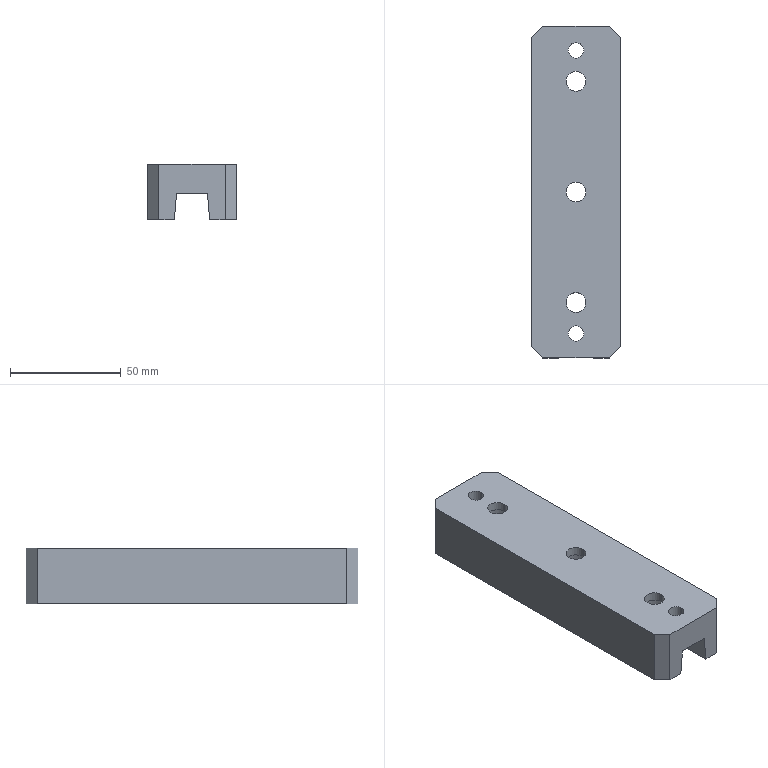Part | Creo | 1 solid | 42 faces | box 40 x 150 x 25 mm | volume 115304 mm3 | plane 26 | cylinder 16 | commonest cylinder face diameters 9 x6 15 x6 7 x4
STEP:
#1=CARTESIAN_POINT('',(0.,0.,0.));
#2=DIRECTION('',(0.,0.,1.));
#3=DIRECTION('',(1.,0.,0.));
#4=AXIS2_PLACEMENT_3D('',#1,#2,#3);
#5=CARTESIAN_POINT('',(-275.949,-119.946,-17.441));
#6=VERTEX_POINT('',#5);
#7=CARTESIAN_POINT('',(-275.949,-164.309,-17.441));
#8=VERTEX_POINT('',#7);
#9=CARTESIAN_POINT('',(-275.949,-119.946,-17.441));
#10=DIRECTION('',(0.,-1.,0.));
#11=VECTOR('',#10,44.362);
#12=LINE('',#9,#11);
#13=EDGE_CURVE('',#6,#8,#12,.T.);
#14=ORIENTED_EDGE('',*,*,#13,.F.);
#15=CARTESIAN_POINT('',(-289.849,-119.946,-17.441));
#16=VERTEX_POINT('',#15);
#17=CARTESIAN_POINT('',(-282.899,-117.127,-17.441));
#18=DIRECTION('',(0.,0.,1.));
#19=DIRECTION('',(-0.9267,-0.3758,0.));
#20=AXIS2_PLACEMENT_3D('',#17,#18,#19);
#21=CIRCLE('',#20,7.5);
#22=EDGE_CURVE('',#16,#6,#21,.T.);
#23=ORIENTED_EDGE('',*,*,#22,.F.);
#24=CARTESIAN_POINT('',(-289.849,-164.309,-17.441));
#25=VERTEX_POINT('',#24);
#26=CARTESIAN_POINT('',(-289.849,-119.946,-17.441));
#27=DIRECTION('',(0.,-1.,0.));
#28=VECTOR('',#27,44.362);
#29=LINE('',#26,#28);
#30=EDGE_CURVE('',#16,#25,#29,.T.);
#31=ORIENTED_EDGE('',*,*,#30,.T.);
#32=CARTESIAN_POINT('',(-282.899,-167.127,-17.441));
#33=DIRECTION('',(0.,0.,1.));
#34=DIRECTION('',(0.9267,0.3758,0.));
#35=AXIS2_PLACEMENT_3D('',#32,#33,#34);
#36=CIRCLE('',#35,7.5);
#37=EDGE_CURVE('',#8,#25,#36,.T.);
#38=ORIENTED_EDGE('',*,*,#37,.F.);
#39=EDGE_LOOP('',(#14,#23,#31,#38));
#40=FACE_OUTER_BOUND('',#39,.F.);
#41=CARTESIAN_POINT('',(-282.899,-167.127,-17.441));
#42=DIRECTION('',(0.,0.,1.));
#43=DIRECTION('',(1.,0.,0.));
#44=AXIS2_PLACEMENT_3D('',#41,#42,#43);
#45=PLANE('',#44);
#46=ADVANCED_FACE('',(#40),#45,.F.);
#47=CARTESIAN_POINT('',(-274.899,-92.127,-29.441));
#48=VERTEX_POINT('',#47);
#49=CARTESIAN_POINT('',(-275.949,-92.127,-17.441));
#50=VERTEX_POINT('',#49);
#51=CARTESIAN_POINT('',(-274.899,-92.127,-29.441));
#52=DIRECTION('',(-0.08716,0.,0.9962));
#53=VECTOR('',#52,12.046);
#54=LINE('',#51,#53);
#55=EDGE_CURVE('',#48,#50,#54,.T.);
#56=ORIENTED_EDGE('',*,*,#55,.T.);
#57=CARTESIAN_POINT('',(-275.949,-114.309,-17.441));
#58=VERTEX_POINT('',#57);
#59=CARTESIAN_POINT('',(-275.949,-92.127,-17.441));
#60=DIRECTION('',(0.,-1.,0.));
#61=VECTOR('',#60,22.181);
#62=LINE('',#59,#61);
#63=EDGE_CURVE('',#50,#58,#62,.T.);
#64=ORIENTED_EDGE('',*,*,#63,.T.);
#65=CARTESIAN_POINT('',(-275.949,-114.309,-17.441));
#66=DIRECTION('',(0.,-1.,0.));
#67=VECTOR('',#66,5.638);
#68=LINE('',#65,#67);
#69=EDGE_CURVE('',#58,#6,#68,.T.);
#70=ORIENTED_EDGE('',*,*,#69,.T.);
#71=ORIENTED_EDGE('',*,*,#13,.T.);
#72=CARTESIAN_POINT('',(-275.949,-169.946,-17.441));
#73=VERTEX_POINT('',#72);
#74=CARTESIAN_POINT('',(-275.949,-164.309,-17.441));
#75=DIRECTION('',(0.,-1.,0.));
#76=VECTOR('',#75,5.638);
#77=LINE('',#74,#76);
#78=EDGE_CURVE('',#8,#73,#77,.T.);
#79=ORIENTED_EDGE('',*,*,#78,.T.);
#80=CARTESIAN_POINT('',(-275.949,-214.309,-17.441));
#81=VERTEX_POINT('',#80);
#82=CARTESIAN_POINT('',(-275.949,-169.946,-17.441));
#83=DIRECTION('',(0.,-1.,0.));
#84=VECTOR('',#83,44.362);
#85=LINE('',#82,#84);
#86=EDGE_CURVE('',#73,#81,#85,.T.);
#87=ORIENTED_EDGE('',*,*,#86,.T.);
#88=CARTESIAN_POINT('',(-275.949,-219.946,-17.441));
#89=VERTEX_POINT('',#88);
#90=CARTESIAN_POINT('',(-275.949,-214.309,-17.441));
#91=DIRECTION('',(0.,-1.,0.));
#92=VECTOR('',#91,5.638);
#93=LINE('',#90,#92);
#94=EDGE_CURVE('',#81,#89,#93,.T.);
#95=ORIENTED_EDGE('',*,*,#94,.T.);
#96=CARTESIAN_POINT('',(-275.949,-242.127,-17.441));
#97=VERTEX_POINT('',#96);
#98=CARTESIAN_POINT('',(-275.949,-219.946,-17.441));
#99=DIRECTION('',(0.,-1.,0.));
#100=VECTOR('',#99,22.181);
#101=LINE('',#98,#100);
#102=EDGE_CURVE('',#89,#97,#101,.T.);
#103=ORIENTED_EDGE('',*,*,#102,.T.);
#104=CARTESIAN_POINT('',(-274.899,-242.127,-29.441));
#105=VERTEX_POINT('',#104);
#106=CARTESIAN_POINT('',(-275.949,-242.127,-17.441));
#107=DIRECTION('',(0.08716,0.,-0.9962));
#108=VECTOR('',#107,12.046);
#109=LINE('',#106,#108);
#110=EDGE_CURVE('',#97,#105,#109,.T.);
#111=ORIENTED_EDGE('',*,*,#110,.T.);
#112=CARTESIAN_POINT('',(-274.899,-92.127,-29.441));
#113=DIRECTION('',(0.,-1.,0.));
#114=VECTOR('',#113,150.);
#115=LINE('',#112,#114);
#116=EDGE_CURVE('',#48,#105,#115,.T.);
#117=ORIENTED_EDGE('',*,*,#116,.F.);
#118=EDGE_LOOP('',(#56,#64,#70,#71,#79,#87,#95,#103,#111,#117));
#119=FACE_OUTER_BOUND('',#118,.F.);
#120=CARTESIAN_POINT('',(-274.899,-92.127,-29.441));
#121=DIRECTION('',(-0.9962,0.,-0.08716));
#122=DIRECTION('',(-0.08716,0.,0.9962));
#123=AXIS2_PLACEMENT_3D('',#120,#121,#122);
#124=PLANE('',#123);
#125=ADVANCED_FACE('',(#119),#124,.T.);
#126=CARTESIAN_POINT('',(-289.849,-92.127,-17.441));
#127=VERTEX_POINT('',#126);
#128=CARTESIAN_POINT('',(-290.899,-92.127,-29.441));
#129=VERTEX_POINT('',#128);
#130=CARTESIAN_POINT('',(-289.849,-92.127,-17.441));
#131=DIRECTION('',(-0.08716,0.,-0.9962));
#132=VECTOR('',#131,12.046);
#133=LINE('',#130,#132);
#134=EDGE_CURVE('',#127,#129,#133,.T.);
#135=ORIENTED_EDGE('',*,*,#134,.F.);
#136=CARTESIAN_POINT('',(-289.849,-92.127,-17.441));
#137=DIRECTION('',(1.,0.,0.));
#138=VECTOR('',#137,13.9);
#139=LINE('',#136,#138);
#140=EDGE_CURVE('',#127,#50,#139,.T.);
#141=ORIENTED_EDGE('',*,*,#140,.T.);
#142=ORIENTED_EDGE('',*,*,#55,.F.);
#143=CARTESIAN_POINT('',(-267.899,-92.127,-29.441));
#144=VERTEX_POINT('',#143);
#145=CARTESIAN_POINT('',(-274.899,-92.127,-29.441));
#146=DIRECTION('',(1.,0.,0.));
#147=VECTOR('',#146,7.);
#148=LINE('',#145,#147);
#149=EDGE_CURVE('',#48,#144,#148,.T.);
#150=ORIENTED_EDGE('',*,*,#149,.T.);
#151=CARTESIAN_POINT('',(-267.899,-92.127,-4.441));
#152=VERTEX_POINT('',#151);
#153=CARTESIAN_POINT('',(-267.899,-92.127,-4.441));
#154=DIRECTION('',(0.,0.,-1.));
#155=VECTOR('',#154,25.);
#156=LINE('',#153,#155);
#157=EDGE_CURVE('',#152,#144,#156,.T.);
#158=ORIENTED_EDGE('',*,*,#157,.F.);
#159=CARTESIAN_POINT('',(-297.899,-92.127,-4.441));
#160=VERTEX_POINT('',#159);
#161=CARTESIAN_POINT('',(-297.899,-92.127,-4.441));
#162=DIRECTION('',(1.,0.,0.));
#163=VECTOR('',#162,30.);
#164=LINE('',#161,#163);
#165=EDGE_CURVE('',#160,#152,#164,.T.);
#166=ORIENTED_EDGE('',*,*,#165,.F.);
#167=CARTESIAN_POINT('',(-297.899,-92.127,-29.441));
#168=VERTEX_POINT('',#167);
#169=CARTESIAN_POINT('',(-297.899,-92.127,-29.441));
#170=DIRECTION('',(0.,0.,1.));
#171=VECTOR('',#170,25.);
#172=LINE('',#169,#171);
#173=EDGE_CURVE('',#168,#160,#172,.T.);
#174=ORIENTED_EDGE('',*,*,#173,.F.);
#175=CARTESIAN_POINT('',(-297.899,-92.127,-29.441));
#176=DIRECTION('',(1.,0.,0.));
#177=VECTOR('',#176,7.);
#178=LINE('',#175,#177);
#179=EDGE_CURVE('',#168,#129,#178,.T.);
#180=ORIENTED_EDGE('',*,*,#179,.T.);
#181=EDGE_LOOP('',(#135,#141,#142,#150,#158,#166,#174,#180));
#182=FACE_OUTER_BOUND('',#181,.F.);
#183=CARTESIAN_POINT('',(-262.899,-92.127,-4.441));
#184=DIRECTION('',(0.,1.,0.));
#185=DIRECTION('',(0.,0.,1.));
#186=AXIS2_PLACEMENT_3D('',#183,#184,#185);
#187=PLANE('',#186);
#188=ADVANCED_FACE('',(#182),#187,.T.);
#189=ORIENTED_EDGE('',*,*,#134,.T.);
#190=CARTESIAN_POINT('',(-290.899,-242.127,-29.441));
#191=VERTEX_POINT('',#190);
#192=CARTESIAN_POINT('',(-290.899,-92.127,-29.441));
#193=DIRECTION('',(0.,-1.,0.));
#194=VECTOR('',#193,150.);
#195=LINE('',#192,#194);
#196=EDGE_CURVE('',#129,#191,#195,.T.);
#197=ORIENTED_EDGE('',*,*,#196,.T.);
#198=CARTESIAN_POINT('',(-289.849,-242.127,-17.441));
#199=VERTEX_POINT('',#198);
#200=CARTESIAN_POINT('',(-290.899,-242.127,-29.441));
#201=DIRECTION('',(0.08716,0.,0.9962));
#202=VECTOR('',#201,12.046);
#203=LINE('',#200,#202);
#204=EDGE_CURVE('',#191,#199,#203,.T.);
#205=ORIENTED_EDGE('',*,*,#204,.T.);
#206=CARTESIAN_POINT('',(-289.849,-219.946,-17.441));
#207=VERTEX_POINT('',#206);
#208=CARTESIAN_POINT('',(-289.849,-219.946,-17.441));
#209=DIRECTION('',(0.,-1.,0.));
#210=VECTOR('',#209,22.181);
#211=LINE('',#208,#210);
#212=EDGE_CURVE('',#207,#199,#211,.T.);
#213=ORIENTED_EDGE('',*,*,#212,.F.);
#214=CARTESIAN_POINT('',(-289.849,-214.309,-17.441));
#215=VERTEX_POINT('',#214);
#216=CARTESIAN_POINT('',(-289.849,-214.309,-17.441));
#217=DIRECTION('',(0.,-1.,0.));
#218=VECTOR('',#217,5.638);
#219=LINE('',#216,#218);
#220=EDGE_CURVE('',#215,#207,#219,.T.);
#221=ORIENTED_EDGE('',*,*,#220,.F.);
#222=CARTESIAN_POINT('',(-289.849,-169.946,-17.441));
#223=VERTEX_POINT('',#222);
#224=CARTESIAN_POINT('',(-289.849,-169.946,-17.441));
#225=DIRECTION('',(0.,-1.,0.));
#226=VECTOR('',#225,44.362);
#227=LINE('',#224,#226);
#228=EDGE_CURVE('',#223,#215,#227,.T.);
#229=ORIENTED_EDGE('',*,*,#228,.F.);
#230=CARTESIAN_POINT('',(-289.849,-164.309,-17.441));
#231=DIRECTION('',(0.,-1.,0.));
#232=VECTOR('',#231,5.638);
#233=LINE('',#230,#232);
#234=EDGE_CURVE('',#25,#223,#233,.T.);
#235=ORIENTED_EDGE('',*,*,#234,.F.);
#236=ORIENTED_EDGE('',*,*,#30,.F.);
#237=CARTESIAN_POINT('',(-289.849,-114.309,-17.441));
#238=VERTEX_POINT('',#237);
#239=CARTESIAN_POINT('',(-289.849,-114.309,-17.441));
#240=DIRECTION('',(0.,-1.,0.));
#241=VECTOR('',#240,5.638);
#242=LINE('',#239,#241);
#243=EDGE_CURVE('',#238,#16,#242,.T.);
#244=ORIENTED_EDGE('',*,*,#243,.F.);
#245=CARTESIAN_POINT('',(-289.849,-92.127,-17.441));
#246=DIRECTION('',(0.,-1.,0.));
#247=VECTOR('',#246,22.181);
#248=LINE('',#245,#247);
#249=EDGE_CURVE('',#127,#238,#248,.T.);
#250=ORIENTED_EDGE('',*,*,#249,.F.);
#251=EDGE_LOOP('',(#189,#197,#205,#213,#221,#229,#235,#236,#244,#250));
#252=FACE_OUTER_BOUND('',#251,.F.);
#253=CARTESIAN_POINT('',(-290.899,-92.127,-29.441));
#254=DIRECTION('',(0.9962,0.,-0.08716));
#255=DIRECTION('',(-0.08716,0.,-0.9962));
#256=AXIS2_PLACEMENT_3D('',#253,#254,#255);
#257=PLANE('',#256);
#258=ADVANCED_FACE('',(#252),#257,.T.);
#259=CARTESIAN_POINT('',(-297.899,-242.127,-29.441));
#260=VERTEX_POINT('',#259);
#261=CARTESIAN_POINT('',(-290.899,-242.127,-29.441));
#262=DIRECTION('',(-1.,0.,0.));
#263=VECTOR('',#262,7.);
#264=LINE('',#261,#263);
#265=EDGE_CURVE('',#191,#260,#264,.T.);
#266=ORIENTED_EDGE('',*,*,#265,.F.);
#267=ORIENTED_EDGE('',*,*,#196,.F.);
#268=ORIENTED_EDGE('',*,*,#179,.F.);
#269=CARTESIAN_POINT('',(-302.899,-97.127,-29.441));
#270=VERTEX_POINT('',#269);
#271=CARTESIAN_POINT('',(-302.899,-97.127,-29.441));
#272=DIRECTION('',(0.7071,0.7071,0.));
#273=VECTOR('',#272,7.071);
#274=LINE('',#271,#273);
#275=EDGE_CURVE('',#270,#168,#274,.T.);
#276=ORIENTED_EDGE('',*,*,#275,.F.);
#277=CARTESIAN_POINT('',(-302.899,-237.127,-29.441));
#278=VERTEX_POINT('',#277);
#279=CARTESIAN_POINT('',(-302.899,-237.127,-29.441));
#280=DIRECTION('',(0.,1.,0.));
#281=VECTOR('',#280,140.);
#282=LINE('',#279,#281);
#283=EDGE_CURVE('',#278,#270,#282,.T.);
#284=ORIENTED_EDGE('',*,*,#283,.F.);
#285=CARTESIAN_POINT('',(-297.899,-242.127,-29.441));
#286=DIRECTION('',(-0.7071,0.7071,0.));
#287=VECTOR('',#286,7.071);
#288=LINE('',#285,#287);
#289=EDGE_CURVE('',#260,#278,#288,.T.);
#290=ORIENTED_EDGE('',*,*,#289,.F.);
#291=EDGE_LOOP('',(#266,#267,#268,#276,#284,#290));
#292=FACE_OUTER_BOUND('',#291,.F.);
#293=CARTESIAN_POINT('',(-302.899,-242.127,-29.441));
#294=DIRECTION('',(0.,0.,1.));
#295=DIRECTION('',(1.,0.,0.));
#296=AXIS2_PLACEMENT_3D('',#293,#294,#295);
#297=PLANE('',#296);
#298=ADVANCED_FACE('',(#292),#297,.F.);
#299=ORIENTED_EDGE('',*,*,#204,.F.);
#300=ORIENTED_EDGE('',*,*,#265,.T.);
#301=CARTESIAN_POINT('',(-297.899,-242.127,-4.441));
#302=VERTEX_POINT('',#301);
#303=CARTESIAN_POINT('',(-297.899,-242.127,-4.441));
#304=DIRECTION('',(0.,0.,-1.));
#305=VECTOR('',#304,25.);
#306=LINE('',#303,#305);
#307=EDGE_CURVE('',#302,#260,#306,.T.);
#308=ORIENTED_EDGE('',*,*,#307,.F.);
#309=CARTESIAN_POINT('',(-267.899,-242.127,-4.441));
#310=VERTEX_POINT('',#309);
#311=CARTESIAN_POINT('',(-267.899,-242.127,-4.441));
#312=DIRECTION('',(-1.,0.,0.));
#313=VECTOR('',#312,30.);
#314=LINE('',#311,#313);
#315=EDGE_CURVE('',#310,#302,#314,.T.);
#316=ORIENTED_EDGE('',*,*,#315,.F.);
#317=CARTESIAN_POINT('',(-267.899,-242.127,-29.441));
#318=VERTEX_POINT('',#317);
#319=CARTESIAN_POINT('',(-267.899,-242.127,-29.441));
#320=DIRECTION('',(0.,0.,1.));
#321=VECTOR('',#320,25.);
#322=LINE('',#319,#321);
#323=EDGE_CURVE('',#318,#310,#322,.T.);
#324=ORIENTED_EDGE('',*,*,#323,.F.);
#325=CARTESIAN_POINT('',(-267.899,-242.127,-29.441));
#326=DIRECTION('',(-1.,0.,0.));
#327=VECTOR('',#326,7.);
#328=LINE('',#325,#327);
#329=EDGE_CURVE('',#318,#105,#328,.T.);
#330=ORIENTED_EDGE('',*,*,#329,.T.);
#331=ORIENTED_EDGE('',*,*,#110,.F.);
#332=CARTESIAN_POINT('',(-275.949,-242.127,-17.441));
#333=DIRECTION('',(-1.,0.,0.));
#334=VECTOR('',#333,13.9);
#335=LINE('',#332,#334);
#336=EDGE_CURVE('',#97,#199,#335,.T.);
#337=ORIENTED_EDGE('',*,*,#336,.T.);
#338=EDGE_LOOP('',(#299,#300,#308,#316,#324,#330,#331,#337));
#339=FACE_OUTER_BOUND('',#338,.F.);
#340=CARTESIAN_POINT('',(-302.899,-242.127,-4.441));
#341=DIRECTION('',(0.,-1.,0.));
#342=DIRECTION('',(0.,0.,-1.));
#343=AXIS2_PLACEMENT_3D('',#340,#341,#342);
#344=PLANE('',#343);
#345=ADVANCED_FACE('',(#339),#344,.T.);
#346=CARTESIAN_POINT('',(-302.899,-237.127,-4.441));
#347=VERTEX_POINT('',#346);
#348=CARTESIAN_POINT('',(-302.899,-237.127,-4.441));
#349=DIRECTION('',(0.7071,-0.7071,0.));
#350=VECTOR('',#349,7.071);
#351=LINE('',#348,#350);
#352=EDGE_CURVE('',#347,#302,#351,.T.);
#353=ORIENTED_EDGE('',*,*,#352,.T.);
#354=ORIENTED_EDGE('',*,*,#307,.T.);
#355=ORIENTED_EDGE('',*,*,#289,.T.);
#356=CARTESIAN_POINT('',(-302.899,-237.127,-29.441));
#357=DIRECTION('',(0.,0.,1.));
#358=VECTOR('',#357,25.);
#359=LINE('',#356,#358);
#360=EDGE_CURVE('',#278,#347,#359,.T.);
#361=ORIENTED_EDGE('',*,*,#360,.T.);
#362=EDGE_LOOP('',(#353,#354,#355,#361));
#363=FACE_OUTER_BOUND('',#362,.F.);
#364=CARTESIAN_POINT('',(-302.899,-237.127,-4.441));
#365=DIRECTION('',(0.7071,0.7071,0.));
#366=DIRECTION('',(-0.7071,0.7071,0.));
#367=AXIS2_PLACEMENT_3D('',#364,#365,#366);
#368=PLANE('',#367);
#369=ADVANCED_FACE('',(#363),#368,.F.);
#370=CARTESIAN_POINT('',(-302.899,-97.127,-4.441));
#371=VERTEX_POINT('',#370);
#372=CARTESIAN_POINT('',(-302.899,-237.127,-4.441));
#373=DIRECTION('',(0.,1.,0.));
#374=VECTOR('',#373,140.);
#375=LINE('',#372,#374);
#376=EDGE_CURVE('',#347,#371,#375,.T.);
#377=ORIENTED_EDGE('',*,*,#376,.T.);
#378=CARTESIAN_POINT('',(-297.899,-92.127,-4.441));
#379=DIRECTION('',(-0.7071,-0.7071,0.));
#380=VECTOR('',#379,7.071);
#381=LINE('',#378,#380);
#382=EDGE_CURVE('',#160,#371,#381,.T.);
#383=ORIENTED_EDGE('',*,*,#382,.F.);
#384=ORIENTED_EDGE('',*,*,#165,.T.);
#385=CARTESIAN_POINT('',(-262.899,-97.127,-4.441));
#386=VERTEX_POINT('',#385);
#387=CARTESIAN_POINT('',(-262.899,-97.127,-4.441));
#388=DIRECTION('',(-0.7071,0.7071,0.));
#389=VECTOR('',#388,7.071);
#390=LINE('',#387,#389);
#391=EDGE_CURVE('',#386,#152,#390,.T.);
#392=ORIENTED_EDGE('',*,*,#391,.F.);
#393=CARTESIAN_POINT('',(-262.899,-237.127,-4.441));
#394=VERTEX_POINT('',#393);
#395=CARTESIAN_POINT('',(-262.899,-97.127,-4.441));
#396=DIRECTION('',(0.,-1.,0.));
#397=VECTOR('',#396,140.);
#398=LINE('',#395,#397);
#399=EDGE_CURVE('',#386,#394,#398,.T.);
#400=ORIENTED_EDGE('',*,*,#399,.T.);
#401=CARTESIAN_POINT('',(-267.899,-242.127,-4.441));
#402=DIRECTION('',(0.7071,0.7071,0.));
#403=VECTOR('',#402,7.071);
#404=LINE('',#401,#403);
#405=EDGE_CURVE('',#310,#394,#404,.T.);
#406=ORIENTED_EDGE('',*,*,#405,.F.);
#407=ORIENTED_EDGE('',*,*,#315,.T.);
#408=ORIENTED_EDGE('',*,*,#352,.F.);
#409=EDGE_LOOP('',(#377,#383,#384,#392,#400,#406,#407,#408));
#410=FACE_OUTER_BOUND('',#409,.F.);
#411=CARTESIAN_POINT('',(-278.399,-167.127,-4.441));
#412=VERTEX_POINT('',#411);
#413=CARTESIAN_POINT('',(-287.399,-167.127,-4.441));
#414=VERTEX_POINT('',#413);
#415=CARTESIAN_POINT('',(-282.899,-167.127,-4.441));
#416=DIRECTION('',(0.,0.,-1.));
#417=DIRECTION('',(1.,0.,0.));
#418=AXIS2_PLACEMENT_3D('',#415,#416,#417);
#419=CIRCLE('',#418,4.5);
#420=EDGE_CURVE('',#412,#414,#419,.T.);
#421=ORIENTED_EDGE('',*,*,#420,.F.);
#422=CARTESIAN_POINT('',(-282.899,-167.127,-4.441));
#423=DIRECTION('',(0.,0.,-1.));
#424=DIRECTION('',(-1.,0.,0.));
#425=AXIS2_PLACEMENT_3D('',#422,#423,#424);
#426=CIRCLE('',#425,4.5);
#427=EDGE_CURVE('',#414,#412,#426,.T.);
#428=ORIENTED_EDGE('',*,*,#427,.F.);
#429=EDGE_LOOP('',(#421,#428));
#430=FACE_BOUND('',#429,.F.);
#431=CARTESIAN_POINT('',(-278.399,-217.127,-4.441));
#432=VERTEX_POINT('',#431);
#433=CARTESIAN_POINT('',(-287.399,-217.127,-4.441));
#434=VERTEX_POINT('',#433);
#435=CARTESIAN_POINT('',(-282.899,-217.127,-4.441));
#436=DIRECTION('',(0.,0.,-1.));
#437=DIRECTION('',(1.,0.,0.));
#438=AXIS2_PLACEMENT_3D('',#435,#436,#437);
#439=CIRCLE('',#438,4.5);
#440=EDGE_CURVE('',#432,#434,#439,.T.);
#441=ORIENTED_EDGE('',*,*,#440,.F.);
#442=CARTESIAN_POINT('',(-282.899,-217.127,-4.441));
#443=DIRECTION('',(0.,0.,-1.));
#444=DIRECTION('',(-1.,0.,0.));
#445=AXIS2_PLACEMENT_3D('',#442,#443,#444);
#446=CIRCLE('',#445,4.5);
#447=EDGE_CURVE('',#434,#432,#446,.T.);
#448=ORIENTED_EDGE('',*,*,#447,.F.);
#449=EDGE_LOOP('',(#441,#448));
#450=FACE_BOUND('',#449,.F.);
#451=CARTESIAN_POINT('',(-279.399,-103.127,-4.441));
#452=VERTEX_POINT('',#451);
#453=CARTESIAN_POINT('',(-286.399,-103.127,-4.441));
#454=VERTEX_POINT('',#453);
#455=CARTESIAN_POINT('',(-282.899,-103.127,-4.441));
#456=DIRECTION('',(0.,0.,-1.));
#457=DIRECTION('',(1.,0.,0.));
#458=AXIS2_PLACEMENT_3D('',#455,#456,#457);
#459=CIRCLE('',#458,3.5);
#460=EDGE_CURVE('',#452,#454,#459,.T.);
#461=ORIENTED_EDGE('',*,*,#460,.F.);
#462=CARTESIAN_POINT('',(-282.899,-103.127,-4.441));
#463=DIRECTION('',(0.,0.,-1.));
#464=DIRECTION('',(-1.,0.,0.));
#465=AXIS2_PLACEMENT_3D('',#462,#463,#464);
#466=CIRCLE('',#465,3.5);
#467=EDGE_CURVE('',#454,#452,#466,.T.);
#468=ORIENTED_EDGE('',*,*,#467,.F.);
#469=EDGE_LOOP('',(#461,#468));
#470=FACE_BOUND('',#469,.F.);
#471=CARTESIAN_POINT('',(-278.399,-117.127,-4.441));
#472=VERTEX_POINT('',#471);
#473=CARTESIAN_POINT('',(-287.399,-117.127,-4.441));
#474=VERTEX_POINT('',#473);
#475=CARTESIAN_POINT('',(-282.899,-117.127,-4.441));
#476=DIRECTION('',(0.,0.,-1.));
#477=DIRECTION('',(1.,0.,0.));
#478=AXIS2_PLACEMENT_3D('',#475,#476,#477);
#479=CIRCLE('',#478,4.5);
#480=EDGE_CURVE('',#472,#474,#479,.T.);
#481=ORIENTED_EDGE('',*,*,#480,.F.);
#482=CARTESIAN_POINT('',(-282.899,-117.127,-4.441));
#483=DIRECTION('',(0.,0.,-1.));
#484=DIRECTION('',(-1.,0.,0.));
#485=AXIS2_PLACEMENT_3D('',#482,#483,#484);
#486=CIRCLE('',#485,4.5);
#487=EDGE_CURVE('',#474,#472,#486,.T.);
#488=ORIENTED_EDGE('',*,*,#487,.F.);
#489=EDGE_LOOP('',(#481,#488));
#490=FACE_BOUND('',#489,.F.);
#491=CARTESIAN_POINT('',(-279.399,-231.127,-4.441));
#492=VERTEX_POINT('',#491);
#493=CARTESIAN_POINT('',(-286.399,-231.127,-4.441));
#494=VERTEX_POINT('',#493);
#495=CARTESIAN_POINT('',(-282.899,-231.127,-4.441));
#496=DIRECTION('',(0.,0.,-1.));
#497=DIRECTION('',(1.,0.,0.));
#498=AXIS2_PLACEMENT_3D('',#495,#496,#497);
#499=CIRCLE('',#498,3.5);
#500=EDGE_CURVE('',#492,#494,#499,.T.);
#501=ORIENTED_EDGE('',*,*,#500,.F.);
#502=CARTESIAN_POINT('',(-282.899,-231.127,-4.441));
#503=DIRECTION('',(0.,0.,-1.));
#504=DIRECTION('',(-1.,0.,0.));
#505=AXIS2_PLACEMENT_3D('',#502,#503,#504);
#506=CIRCLE('',#505,3.5);
#507=EDGE_CURVE('',#494,#492,#506,.T.);
#508=ORIENTED_EDGE('',*,*,#507,.F.);
#509=EDGE_LOOP('',(#501,#508));
#510=FACE_BOUND('',#509,.F.);
#511=CARTESIAN_POINT('',(-302.899,-242.127,-4.441));
#512=DIRECTION('',(0.,0.,1.));
#513=DIRECTION('',(1.,0.,0.));
#514=AXIS2_PLACEMENT_3D('',#511,#512,#513);
#515=PLANE('',#514);
#516=ADVANCED_FACE('',(#410,#430,#450,#470,#490,#510),#515,.T.);
#517=ORIENTED_EDGE('',*,*,#480,.T.);
#518=CARTESIAN_POINT('',(-287.399,-117.127,-8.441));
#519=VERTEX_POINT('',#518);
#520=CARTESIAN_POINT('',(-287.399,-117.127,-4.441));
#521=DIRECTION('',(0.,0.,-1.));
#522=VECTOR('',#521,4.);
#523=LINE('',#520,#522);
#524=EDGE_CURVE('',#474,#519,#523,.T.);
#525=ORIENTED_EDGE('',*,*,#524,.T.);
#526=CARTESIAN_POINT('',(-278.399,-117.127,-8.441));
#527=VERTEX_POINT('',#526);
#528=CARTESIAN_POINT('',(-282.899,-117.127,-8.441));
#529=DIRECTION('',(0.,0.,1.));
#530=DIRECTION('',(-1.,0.,0.));
#531=AXIS2_PLACEMENT_3D('',#528,#529,#530);
#532=CIRCLE('',#531,4.5);
#533=EDGE_CURVE('',#519,#527,#532,.T.);
#534=ORIENTED_EDGE('',*,*,#533,.T.);
#535=CARTESIAN_POINT('',(-278.399,-117.127,-4.441));
#536=DIRECTION('',(0.,0.,-1.));
#537=VECTOR('',#536,4.);
#538=LINE('',#535,#537);
#539=EDGE_CURVE('',#472,#527,#538,.T.);
#540=ORIENTED_EDGE('',*,*,#539,.F.);
#541=EDGE_LOOP('',(#517,#525,#534,#540));
#542=FACE_OUTER_BOUND('',#541,.F.);
#543=CARTESIAN_POINT('',(-282.899,-117.127,26.559));
#544=DIRECTION('',(0.,0.,-1.));
#545=DIRECTION('',(-1.,0.,0.));
#546=AXIS2_PLACEMENT_3D('',#543,#544,#545);
#547=CYLINDRICAL_SURFACE('',#546,4.5);
#548=ADVANCED_FACE('',(#542),#547,.F.);
#549=ORIENTED_EDGE('',*,*,#487,.T.);
#550=ORIENTED_EDGE('',*,*,#539,.T.);
#551=CARTESIAN_POINT('',(-282.899,-117.127,-8.441));
#552=DIRECTION('',(0.,0.,1.));
#553=DIRECTION('',(1.,0.,0.));
#554=AXIS2_PLACEMENT_3D('',#551,#552,#553);
#555=CIRCLE('',#554,4.5);
#556=EDGE_CURVE('',#527,#519,#555,.T.);
#557=ORIENTED_EDGE('',*,*,#556,.T.);
#558=ORIENTED_EDGE('',*,*,#524,.F.);
#559=EDGE_LOOP('',(#549,#550,#557,#558));
#560=FACE_OUTER_BOUND('',#559,.F.);
#561=CARTESIAN_POINT('',(-282.899,-117.127,26.559));
#562=DIRECTION('',(0.,0.,-1.));
#563=DIRECTION('',(-1.,0.,0.));
#564=AXIS2_PLACEMENT_3D('',#561,#562,#563);
#565=CYLINDRICAL_SURFACE('',#564,4.5);
#566=ADVANCED_FACE('',(#560),#565,.F.);
#567=CARTESIAN_POINT('',(-290.399,-117.127,-8.441));
#568=VERTEX_POINT('',#567);
#569=CARTESIAN_POINT('',(-275.399,-117.127,-8.441));
#570=VERTEX_POINT('',#569);
#571=CARTESIAN_POINT('',(-282.899,-117.127,-8.441));
#572=DIRECTION('',(0.,0.,-1.));
#573=DIRECTION('',(-1.,0.,0.));
#574=AXIS2_PLACEMENT_3D('',#571,#572,#573);
#575=CIRCLE('',#574,7.5);
#576=EDGE_CURVE('',#568,#570,#575,.T.);
#577=ORIENTED_EDGE('',*,*,#576,.F.);
#578=CARTESIAN_POINT('',(-282.899,-117.127,-8.441));
#579=DIRECTION('',(0.,0.,-1.));
#580=DIRECTION('',(1.,0.,0.));
#581=AXIS2_PLACEMENT_3D('',#578,#579,#580);
#582=CIRCLE('',#581,7.5);
#583=EDGE_CURVE('',#570,#568,#582,.T.);
#584=ORIENTED_EDGE('',*,*,#583,.F.);
#585=EDGE_LOOP('',(#577,#584));
#586=FACE_OUTER_BOUND('',#585,.F.);
#587=ORIENTED_EDGE('',*,*,#533,.F.);
#588=ORIENTED_EDGE('',*,*,#556,.F.);
#589=EDGE_LOOP('',(#587,#588));
#590=FACE_BOUND('',#589,.F.);
#591=CARTESIAN_POINT('',(-282.899,-117.127,-8.441));
#592=DIRECTION('',(0.,0.,-1.));
#593=DIRECTION('',(-1.,0.,0.));
#594=AXIS2_PLACEMENT_3D('',#591,#592,#593);
#595=PLANE('',#594);
#596=ADVANCED_FACE('',(#586,#590),#595,.T.);
#597=ORIENTED_EDGE('',*,*,#576,.T.);
#598=CARTESIAN_POINT('',(-275.399,-117.127,-17.441));
#599=VERTEX_POINT('',#598);
#600=CARTESIAN_POINT('',(-275.399,-117.127,-8.441));
#601=DIRECTION('',(0.,0.,-1.));
#602=VECTOR('',#601,9.);
#603=LINE('',#600,#602);
#604=EDGE_CURVE('',#570,#599,#603,.T.);
#605=ORIENTED_EDGE('',*,*,#604,.T.);
#606=CARTESIAN_POINT('',(-282.899,-117.127,-17.441));
#607=DIRECTION('',(0.,0.,1.));
#608=DIRECTION('',(1.,0.,0.));
#609=AXIS2_PLACEMENT_3D('',#606,#607,#608);
#610=CIRCLE('',#609,7.5);
#611=EDGE_CURVE('',#599,#58,#610,.T.);
#612=ORIENTED_EDGE('',*,*,#611,.T.);
#613=CARTESIAN_POINT('',(-282.899,-117.127,-17.441));
#614=DIRECTION('',(0.,0.,1.));
#615=DIRECTION('',(0.9267,0.3758,0.));
#616=AXIS2_PLACEMENT_3D('',#613,#614,#615);
#617=CIRCLE('',#616,7.5);
#618=EDGE_CURVE('',#58,#238,#617,.T.);
#619=ORIENTED_EDGE('',*,*,#618,.T.);
#620=CARTESIAN_POINT('',(-290.399,-117.127,-17.441));
#621=VERTEX_POINT('',#620);
#622=CARTESIAN_POINT('',(-282.899,-117.127,-17.441));
#623=DIRECTION('',(0.,0.,1.));
#624=DIRECTION('',(-0.9267,0.3758,0.));
#625=AXIS2_PLACEMENT_3D('',#622,#623,#624);
#626=CIRCLE('',#625,7.5);
#627=EDGE_CURVE('',#238,#621,#626,.T.);
#628=ORIENTED_EDGE('',*,*,#627,.T.);
#629=CARTESIAN_POINT('',(-290.399,-117.127,-8.441));
#630=DIRECTION('',(0.00000035,0.,-1.));
#631=VECTOR('',#630,9.);
#632=LINE('',#629,#631);
#633=EDGE_CURVE('',#568,#621,#632,.T.);
#634=ORIENTED_EDGE('',*,*,#633,.F.);
#635=EDGE_LOOP('',(#597,#605,#612,#619,#628,#634));
#636=FACE_OUTER_BOUND('',#635,.F.);
#637=CARTESIAN_POINT('',(-282.899,-117.127,-8.441));
#638=DIRECTION('',(0.,0.,-1.));
#639=DIRECTION('',(-1.,0.,0.));
#640=AXIS2_PLACEMENT_3D('',#637,#638,#639);
#641=CYLINDRICAL_SURFACE('',#640,7.5);
#642=ADVANCED_FACE('',(#636),#641,.F.);
#643=ORIENTED_EDGE('',*,*,#583,.T.);
#644=ORIENTED_EDGE('',*,*,#633,.T.);
#645=CARTESIAN_POINT('',(-282.899,-117.127,-17.441));
#646=DIRECTION('',(0.,0.,1.));
#647=DIRECTION('',(-1.,0.,0.));
#648=AXIS2_PLACEMENT_3D('',#645,#646,#647);
#649=CIRCLE('',#648,7.5);
#650=EDGE_CURVE('',#621,#16,#649,.T.);
#651=ORIENTED_EDGE('',*,*,#650,.T.);
#652=ORIENTED_EDGE('',*,*,#22,.T.);
#653=CARTESIAN_POINT('',(-282.899,-117.127,-17.441));
#654=DIRECTION('',(0.,0.,1.));
#655=DIRECTION('',(0.9267,-0.3758,0.));
#656=AXIS2_PLACEMENT_3D('',#653,#654,#655);
#657=CIRCLE('',#656,7.5);
#658=EDGE_CURVE('',#6,#599,#657,.T.);
#659=ORIENTED_EDGE('',*,*,#658,.T.);
#660=ORIENTED_EDGE('',*,*,#604,.F.);
#661=EDGE_LOOP('',(#643,#644,#651,#652,#659,#660));
#662=FACE_OUTER_BOUND('',#661,.F.);
#663=CARTESIAN_POINT('',(-282.899,-117.127,-8.441));
#664=DIRECTION('',(0.,0.,-1.));
#665=DIRECTION('',(-1.,0.,0.));
#666=AXIS2_PLACEMENT_3D('',#663,#664,#665);
#667=CYLINDRICAL_SURFACE('',#666,7.5);
#668=ADVANCED_FACE('',(#662),#667,.F.);
#669=ORIENTED_EDGE('',*,*,#650,.F.);
#670=ORIENTED_EDGE('',*,*,#627,.F.);
#671=ORIENTED_EDGE('',*,*,#243,.T.);
#672=EDGE_LOOP('',(#669,#670,#671));
#673=FACE_OUTER_BOUND('',#672,.F.);
#674=CARTESIAN_POINT('',(-282.899,-117.127,-17.441));
#675=DIRECTION('',(0.,0.,-1.));
#676=DIRECTION('',(-1.,0.,0.));
#677=AXIS2_PLACEMENT_3D('',#674,#675,#676);
#678=PLANE('',#677);
#679=ADVANCED_FACE('',(#673),#678,.F.);
#680=ORIENTED_EDGE('',*,*,#658,.F.);
#681=ORIENTED_EDGE('',*,*,#69,.F.);
#682=ORIENTED_EDGE('',*,*,#611,.F.);
#683=EDGE_LOOP('',(#680,#681,#682));
#684=FACE_OUTER_BOUND('',#683,.F.);
#685=CARTESIAN_POINT('',(-282.899,-117.127,-17.441));
#686=DIRECTION('',(0.,0.,-1.));
#687=DIRECTION('',(-1.,0.,0.));
#688=AXIS2_PLACEMENT_3D('',#685,#686,#687);
#689=PLANE('',#688);
#690=ADVANCED_FACE('',(#684),#689,.F.);
#691=ORIENTED_EDGE('',*,*,#249,.T.);
#692=ORIENTED_EDGE('',*,*,#618,.F.);
#693=ORIENTED_EDGE('',*,*,#63,.F.);
#694=ORIENTED_EDGE('',*,*,#140,.F.);
#695=EDGE_LOOP('',(#691,#692,#693,#694));
#696=FACE_OUTER_BOUND('',#695,.F.);
#697=CARTESIAN_POINT('',(-279.399,-103.127,-17.441));
#698=VERTEX_POINT('',#697);
#699=CARTESIAN_POINT('',(-286.399,-103.127,-17.441));
#700=VERTEX_POINT('',#699);
#701=CARTESIAN_POINT('',(-282.899,-103.127,-17.441));
#702=DIRECTION('',(0.,0.,1.));
#703=DIRECTION('',(1.,0.,0.));
#704=AXIS2_PLACEMENT_3D('',#701,#702,#703);
#705=CIRCLE('',#704,3.5);
#706=EDGE_CURVE('',#698,#700,#705,.T.);
#707=ORIENTED_EDGE('',*,*,#706,.F.);
#708=CARTESIAN_POINT('',(-282.899,-103.127,-17.441));
#709=DIRECTION('',(0.,0.,1.));
#710=DIRECTION('',(-1.,0.,0.));
#711=AXIS2_PLACEMENT_3D('',#708,#709,#710);
#712=CIRCLE('',#711,3.5);
#713=EDGE_CURVE('',#700,#698,#712,.T.);
#714=ORIENTED_EDGE('',*,*,#713,.F.);
#715=EDGE_LOOP('',(#707,#714));
#716=FACE_BOUND('',#715,.F.);
#717=CARTESIAN_POINT('',(-282.899,-167.127,-17.441));
#718=DIRECTION('',(0.,0.,1.));
#719=DIRECTION('',(1.,0.,0.));
#720=AXIS2_PLACEMENT_3D('',#717,#718,#719);
#721=PLANE('',#720);
#722=ADVANCED_FACE('',(#696,#716),#721,.F.);
#723=ORIENTED_EDGE('',*,*,#467,.T.);
#724=CARTESIAN_POINT('',(-279.399,-103.127,-17.441));
#725=DIRECTION('',(0.,0.,1.));
#726=VECTOR('',#725,13.);
#727=LINE('',#724,#726);
#728=EDGE_CURVE('',#698,#452,#727,.T.);
#729=ORIENTED_EDGE('',*,*,#728,.F.);
#730=ORIENTED_EDGE('',*,*,#706,.T.);
#731=CARTESIAN_POINT('',(-286.399,-103.127,-17.441));
#732=DIRECTION('',(0.,0.,1.));
#733=VECTOR('',#732,13.);
#734=LINE('',#731,#733);
#735=EDGE_CURVE('',#700,#454,#734,.T.);
#736=ORIENTED_EDGE('',*,*,#735,.T.);
#737=EDGE_LOOP('',(#723,#729,#730,#736));
#738=FACE_OUTER_BOUND('',#737,.F.);
#739=CARTESIAN_POINT('',(-282.899,-103.127,-140.441));
#740=DIRECTION('',(0.,0.,1.));
#741=DIRECTION('',(1.,0.,0.));
#742=AXIS2_PLACEMENT_3D('',#739,#740,#741);
#743=CYLINDRICAL_SURFACE('',#742,3.5);
#744=ADVANCED_FACE('',(#738),#743,.F.);
#745=ORIENTED_EDGE('',*,*,#460,.T.);
#746=ORIENTED_EDGE('',*,*,#735,.F.);
#747=ORIENTED_EDGE('',*,*,#713,.T.);
#748=ORIENTED_EDGE('',*,*,#728,.T.);
#749=EDGE_LOOP('',(#745,#746,#747,#748));
#750=FACE_OUTER_BOUND('',#749,.F.);
#751=CARTESIAN_POINT('',(-282.899,-103.127,-140.441));
#752=DIRECTION('',(0.,0.,1.));
#753=DIRECTION('',(1.,0.,0.));
#754=AXIS2_PLACEMENT_3D('',#751,#752,#753);
#755=CYLINDRICAL_SURFACE('',#754,3.5);
#756=ADVANCED_FACE('',(#750),#755,.F.);
#757=ORIENTED_EDGE('',*,*,#420,.T.);
#758=CARTESIAN_POINT('',(-287.399,-167.127,-8.441));
#759=VERTEX_POINT('',#758);
#760=CARTESIAN_POINT('',(-287.399,-167.127,-4.441));
#761=DIRECTION('',(0.,0.,-1.));
#762=VECTOR('',#761,4.);
#763=LINE('',#760,#762);
#764=EDGE_CURVE('',#414,#759,#763,.T.);
#765=ORIENTED_EDGE('',*,*,#764,.T.);
#766=CARTESIAN_POINT('',(-278.399,-167.127,-8.441));
#767=VERTEX_POINT('',#766);
#768=CARTESIAN_POINT('',(-282.899,-167.127,-8.441));
#769=DIRECTION('',(0.,0.,1.));
#770=DIRECTION('',(-1.,0.,0.));
#771=AXIS2_PLACEMENT_3D('',#768,#769,#770);
#772=CIRCLE('',#771,4.5);
#773=EDGE_CURVE('',#759,#767,#772,.T.);
#774=ORIENTED_EDGE('',*,*,#773,.T.);
#775=CARTESIAN_POINT('',(-278.399,-167.127,-4.441));
#776=DIRECTION('',(0.,0.,-1.));
#777=VECTOR('',#776,4.);
#778=LINE('',#775,#777);
#779=EDGE_CURVE('',#412,#767,#778,.T.);
#780=ORIENTED_EDGE('',*,*,#779,.F.);
#781=EDGE_LOOP('',(#757,#765,#774,#780));
#782=FACE_OUTER_BOUND('',#781,.F.);
#783=CARTESIAN_POINT('',(-282.899,-167.127,26.559));
#784=DIRECTION('',(0.,0.,-1.));
#785=DIRECTION('',(-1.,0.,0.));
#786=AXIS2_PLACEMENT_3D('',#783,#784,#785);
#787=CYLINDRICAL_SURFACE('',#786,4.5);
#788=ADVANCED_FACE('',(#782),#787,.F.);
#789=ORIENTED_EDGE('',*,*,#427,.T.);
#790=ORIENTED_EDGE('',*,*,#779,.T.);
#791=CARTESIAN_POINT('',(-282.899,-167.127,-8.441));
#792=DIRECTION('',(0.,0.,1.));
#793=DIRECTION('',(1.,0.,0.));
#794=AXIS2_PLACEMENT_3D('',#791,#792,#793);
#795=CIRCLE('',#794,4.5);
#796=EDGE_CURVE('',#767,#759,#795,.T.);
#797=ORIENTED_EDGE('',*,*,#796,.T.);
#798=ORIENTED_EDGE('',*,*,#764,.F.);
#799=EDGE_LOOP('',(#789,#790,#797,#798));
#800=FACE_OUTER_BOUND('',#799,.F.);
#801=CARTESIAN_POINT('',(-282.899,-167.127,26.559));
#802=DIRECTION('',(0.,0.,-1.));
#803=DIRECTION('',(-1.,0.,0.));
#804=AXIS2_PLACEMENT_3D('',#801,#802,#803);
#805=CYLINDRICAL_SURFACE('',#804,4.5);
#806=ADVANCED_FACE('',(#800),#805,.F.);
#807=CARTESIAN_POINT('',(-290.399,-167.127,-8.441));
#808=VERTEX_POINT('',#807);
#809=CARTESIAN_POINT('',(-275.399,-167.127,-8.441));
#810=VERTEX_POINT('',#809);
#811=CARTESIAN_POINT('',(-282.899,-167.127,-8.441));
#812=DIRECTION('',(0.,0.,-1.));
#813=DIRECTION('',(-1.,0.,0.));
#814=AXIS2_PLACEMENT_3D('',#811,#812,#813);
#815=CIRCLE('',#814,7.5);
#816=EDGE_CURVE('',#808,#810,#815,.T.);
#817=ORIENTED_EDGE('',*,*,#816,.F.);
#818=CARTESIAN_POINT('',(-282.899,-167.127,-8.441));
#819=DIRECTION('',(0.,0.,-1.));
#820=DIRECTION('',(1.,0.,0.));
#821=AXIS2_PLACEMENT_3D('',#818,#819,#820);
#822=CIRCLE('',#821,7.5);
#823=EDGE_CURVE('',#810,#808,#822,.T.);
#824=ORIENTED_EDGE('',*,*,#823,.F.);
#825=EDGE_LOOP('',(#817,#824));
#826=FACE_OUTER_BOUND('',#825,.F.);
#827=ORIENTED_EDGE('',*,*,#773,.F.);
#828=ORIENTED_EDGE('',*,*,#796,.F.);
#829=EDGE_LOOP('',(#827,#828));
#830=FACE_BOUND('',#829,.F.);
#831=CARTESIAN_POINT('',(-282.899,-167.127,-8.441));
#832=DIRECTION('',(0.,0.,-1.));
#833=DIRECTION('',(-1.,0.,0.));
#834=AXIS2_PLACEMENT_3D('',#831,#832,#833);
#835=PLANE('',#834);
#836=ADVANCED_FACE('',(#826,#830),#835,.T.);
#837=ORIENTED_EDGE('',*,*,#816,.T.);
#838=CARTESIAN_POINT('',(-275.399,-167.127,-17.441));
#839=VERTEX_POINT('',#838);
#840=CARTESIAN_POINT('',(-275.399,-167.127,-8.441));
#841=DIRECTION('',(0.,0.,-1.));
#842=VECTOR('',#841,9.);
#843=LINE('',#840,#842);
#844=EDGE_CURVE('',#810,#839,#843,.T.);
#845=ORIENTED_EDGE('',*,*,#844,.T.);
#846=CARTESIAN_POINT('',(-282.899,-167.127,-17.441));
#847=DIRECTION('',(0.,0.,1.));
#848=DIRECTION('',(1.,0.,0.));
#849=AXIS2_PLACEMENT_3D('',#846,#847,#848);
#850=CIRCLE('',#849,7.5);
#851=EDGE_CURVE('',#839,#8,#850,.T.);
#852=ORIENTED_EDGE('',*,*,#851,.T.);
#853=ORIENTED_EDGE('',*,*,#37,.T.);
#854=CARTESIAN_POINT('',(-290.399,-167.127,-17.441));
#855=VERTEX_POINT('',#854);
#856=CARTESIAN_POINT('',(-282.899,-167.127,-17.441));
#857=DIRECTION('',(0.,0.,1.));
#858=DIRECTION('',(-0.9267,0.3758,0.));
#859=AXIS2_PLACEMENT_3D('',#856,#857,#858);
#860=CIRCLE('',#859,7.5);
#861=EDGE_CURVE('',#25,#855,#860,.T.);
#862=ORIENTED_EDGE('',*,*,#861,.T.);
#863=CARTESIAN_POINT('',(-290.399,-167.127,-8.441));
#864=DIRECTION('',(0.00000035,0.,-1.));
#865=VECTOR('',#864,9.);
#866=LINE('',#863,#865);
#867=EDGE_CURVE('',#808,#855,#866,.T.);
#868=ORIENTED_EDGE('',*,*,#867,.F.);
#869=EDGE_LOOP('',(#837,#845,#852,#853,#862,#868));
#870=FACE_OUTER_BOUND('',#869,.F.);
#871=CARTESIAN_POINT('',(-282.899,-167.127,-8.441));
#872=DIRECTION('',(0.,0.,-1.));
#873=DIRECTION('',(-1.,0.,0.));
#874=AXIS2_PLACEMENT_3D('',#871,#872,#873);
#875=CYLINDRICAL_SURFACE('',#874,7.5);
#876=ADVANCED_FACE('',(#870),#875,.F.);
#877=ORIENTED_EDGE('',*,*,#823,.T.);
#878=ORIENTED_EDGE('',*,*,#867,.T.);
#879=CARTESIAN_POINT('',(-282.899,-167.127,-17.441));
#880=DIRECTION('',(0.,0.,1.));
#881=DIRECTION('',(-1.,0.,0.));
#882=AXIS2_PLACEMENT_3D('',#879,#880,#881);
#883=CIRCLE('',#882,7.5);
#884=EDGE_CURVE('',#855,#223,#883,.T.);
#885=ORIENTED_EDGE('',*,*,#884,.T.);
#886=CARTESIAN_POINT('',(-282.899,-167.127,-17.441));
#887=DIRECTION('',(0.,0.,1.));
#888=DIRECTION('',(-0.9267,-0.3758,0.));
#889=AXIS2_PLACEMENT_3D('',#886,#887,#888);
#890=CIRCLE('',#889,7.5);
#891=EDGE_CURVE('',#223,#73,#890,.T.);
#892=ORIENTED_EDGE('',*,*,#891,.T.);
#893=CARTESIAN_POINT('',(-282.899,-167.127,-17.441));
#894=DIRECTION('',(0.,0.,1.));
#895=DIRECTION('',(0.9267,-0.3758,0.));
#896=AXIS2_PLACEMENT_3D('',#893,#894,#895);
#897=CIRCLE('',#896,7.5);
#898=EDGE_CURVE('',#73,#839,#897,.T.);
#899=ORIENTED_EDGE('',*,*,#898,.T.);
#900=ORIENTED_EDGE('',*,*,#844,.F.);
#901=EDGE_LOOP('',(#877,#878,#885,#892,#899,#900));
#902=FACE_OUTER_BOUND('',#901,.F.);
#903=CARTESIAN_POINT('',(-282.899,-167.127,-8.441));
#904=DIRECTION('',(0.,0.,-1.));
#905=DIRECTION('',(-1.,0.,0.));
#906=AXIS2_PLACEMENT_3D('',#903,#904,#905);
#907=CYLINDRICAL_SURFACE('',#906,7.5);
#908=ADVANCED_FACE('',(#902),#907,.F.);
#909=ORIENTED_EDGE('',*,*,#884,.F.);
#910=ORIENTED_EDGE('',*,*,#861,.F.);
#911=ORIENTED_EDGE('',*,*,#234,.T.);
#912=EDGE_LOOP('',(#909,#910,#911));
#913=FACE_OUTER_BOUND('',#912,.F.);
#914=CARTESIAN_POINT('',(-282.899,-167.127,-17.441));
#915=DIRECTION('',(0.,0.,-1.));
#916=DIRECTION('',(-1.,0.,0.));
#917=AXIS2_PLACEMENT_3D('',#914,#915,#916);
#918=PLANE('',#917);
#919=ADVANCED_FACE('',(#913),#918,.F.);
#920=ORIENTED_EDGE('',*,*,#86,.F.);
#921=ORIENTED_EDGE('',*,*,#891,.F.);
#922=ORIENTED_EDGE('',*,*,#228,.T.);
#923=CARTESIAN_POINT('',(-282.899,-217.127,-17.441));
#924=DIRECTION('',(0.,0.,1.));
#925=DIRECTION('',(0.9267,0.3758,0.));
#926=AXIS2_PLACEMENT_3D('',#923,#924,#925);
#927=CIRCLE('',#926,7.5);
#928=EDGE_CURVE('',#81,#215,#927,.T.);
#929=ORIENTED_EDGE('',*,*,#928,.F.);
#930=EDGE_LOOP('',(#920,#921,#922,#929));
#931=FACE_OUTER_BOUND('',#930,.F.);
#932=CARTESIAN_POINT('',(-282.899,-167.127,-17.441));
#933=DIRECTION('',(0.,0.,1.));
#934=DIRECTION('',(1.,0.,0.));
#935=AXIS2_PLACEMENT_3D('',#932,#933,#934);
#936=PLANE('',#935);
#937=ADVANCED_FACE('',(#931),#936,.F.);
#938=CARTESIAN_POINT('',(-290.399,-217.127,-8.441));
#939=VERTEX_POINT('',#938);
#940=CARTESIAN_POINT('',(-275.399,-217.127,-8.441));
#941=VERTEX_POINT('',#940);
#942=CARTESIAN_POINT('',(-282.899,-217.127,-8.441));
#943=DIRECTION('',(0.,0.,-1.));
#944=DIRECTION('',(-1.,0.,0.));
#945=AXIS2_PLACEMENT_3D('',#942,#943,#944);
#946=CIRCLE('',#945,7.5);
#947=EDGE_CURVE('',#939,#941,#946,.T.);
#948=ORIENTED_EDGE('',*,*,#947,.T.);
#949=CARTESIAN_POINT('',(-275.399,-217.127,-17.441));
#950=VERTEX_POINT('',#949);
#951=CARTESIAN_POINT('',(-275.399,-217.127,-8.441));
#952=DIRECTION('',(0.,0.,-1.));
#953=VECTOR('',#952,9.);
#954=LINE('',#951,#953);
#955=EDGE_CURVE('',#941,#950,#954,.T.);
#956=ORIENTED_EDGE('',*,*,#955,.T.);
#957=CARTESIAN_POINT('',(-282.899,-217.127,-17.441));
#958=DIRECTION('',(0.,0.,1.));
#959=DIRECTION('',(1.,0.,0.));
#960=AXIS2_PLACEMENT_3D('',#957,#958,#959);
#961=CIRCLE('',#960,7.5);
#962=EDGE_CURVE('',#950,#81,#961,.T.);
#963=ORIENTED_EDGE('',*,*,#962,.T.);
#964=ORIENTED_EDGE('',*,*,#928,.T.);
#965=CARTESIAN_POINT('',(-290.399,-217.127,-17.441));
#966=VERTEX_POINT('',#965);
#967=CARTESIAN_POINT('',(-282.899,-217.127,-17.441));
#968=DIRECTION('',(0.,0.,1.));
#969=DIRECTION('',(-0.9267,0.3758,0.));
#970=AXIS2_PLACEMENT_3D('',#967,#968,#969);
#971=CIRCLE('',#970,7.5);
#972=EDGE_CURVE('',#215,#966,#971,.T.);
#973=ORIENTED_EDGE('',*,*,#972,.T.);
#974=CARTESIAN_POINT('',(-290.399,-217.127,-8.441));
#975=DIRECTION('',(0.00000035,0.,-1.));
#976=VECTOR('',#975,9.);
#977=LINE('',#974,#976);
#978=EDGE_CURVE('',#939,#966,#977,.T.);
#979=ORIENTED_EDGE('',*,*,#978,.F.);
#980=EDGE_LOOP('',(#948,#956,#963,#964,#973,#979));
#981=FACE_OUTER_BOUND('',#980,.F.);
#982=CARTESIAN_POINT('',(-282.899,-217.127,-8.441));
#983=DIRECTION('',(0.,0.,-1.));
#984=DIRECTION('',(-1.,0.,0.));
#985=AXIS2_PLACEMENT_3D('',#982,#983,#984);
#986=CYLINDRICAL_SURFACE('',#985,7.5);
#987=ADVANCED_FACE('',(#981),#986,.F.);
#988=ORIENTED_EDGE('',*,*,#947,.F.);
#989=CARTESIAN_POINT('',(-282.899,-217.127,-8.441));
#990=DIRECTION('',(0.,0.,-1.));
#991=DIRECTION('',(1.,0.,0.));
#992=AXIS2_PLACEMENT_3D('',#989,#990,#991);
#993=CIRCLE('',#992,7.5);
#994=EDGE_CURVE('',#941,#939,#993,.T.);
#995=ORIENTED_EDGE('',*,*,#994,.F.);
#996=EDGE_LOOP('',(#988,#995));
#997=FACE_OUTER_BOUND('',#996,.F.);
#998=CARTESIAN_POINT('',(-287.399,-217.127,-8.441));
#999=VERTEX_POINT('',#998);
#1000=CARTESIAN_POINT('',(-278.399,-217.127,-8.441));
#1001=VERTEX_POINT('',#1000);
#1002=CARTESIAN_POINT('',(-282.899,-217.127,-8.441));
#1003=DIRECTION('',(0.,0.,1.));
#1004=DIRECTION('',(-1.,0.,0.));
#1005=AXIS2_PLACEMENT_3D('',#1002,#1003,#1004);
#1006=CIRCLE('',#1005,4.5);
#1007=EDGE_CURVE('',#999,#1001,#1006,.T.);
#1008=ORIENTED_EDGE('',*,*,#1007,.F.);
#1009=CARTESIAN_POINT('',(-282.899,-217.127,-8.441));
#1010=DIRECTION('',(0.,0.,1.));
#1011=DIRECTION('',(1.,0.,0.));
#1012=AXIS2_PLACEMENT_3D('',#1009,#1010,#1011);
#1013=CIRCLE('',#1012,4.5);
#1014=EDGE_CURVE('',#1001,#999,#1013,.T.);
#1015=ORIENTED_EDGE('',*,*,#1014,.F.);
#1016=EDGE_LOOP('',(#1008,#1015));
#1017=FACE_BOUND('',#1016,.F.);
#1018=CARTESIAN_POINT('',(-282.899,-217.127,-8.441));
#1019=DIRECTION('',(0.,0.,-1.));
#1020=DIRECTION('',(-1.,0.,0.));
#1021=AXIS2_PLACEMENT_3D('',#1018,#1019,#1020);
#1022=PLANE('',#1021);
#1023=ADVANCED_FACE('',(#997,#1017),#1022,.T.);
#1024=ORIENTED_EDGE('',*,*,#440,.T.);
#1025=CARTESIAN_POINT('',(-287.399,-217.127,-4.441));
#1026=DIRECTION('',(0.,0.,-1.));
#1027=VECTOR('',#1026,4.);
#1028=LINE('',#1025,#1027);
#1029=EDGE_CURVE('',#434,#999,#1028,.T.);
#1030=ORIENTED_EDGE('',*,*,#1029,.T.);
#1031=ORIENTED_EDGE('',*,*,#1007,.T.);
#1032=CARTESIAN_POINT('',(-278.399,-217.127,-4.441));
#1033=DIRECTION('',(0.,0.,-1.));
#1034=VECTOR('',#1033,4.);
#1035=LINE('',#1032,#1034);
#1036=EDGE_CURVE('',#432,#1001,#1035,.T.);
#1037=ORIENTED_EDGE('',*,*,#1036,.F.);
#1038=EDGE_LOOP('',(#1024,#1030,#1031,#1037));
#1039=FACE_OUTER_BOUND('',#1038,.F.);
#1040=CARTESIAN_POINT('',(-282.899,-217.127,26.559));
#1041=DIRECTION('',(0.,0.,-1.));
#1042=DIRECTION('',(-1.,0.,0.));
#1043=AXIS2_PLACEMENT_3D('',#1040,#1041,#1042);
#1044=CYLINDRICAL_SURFACE('',#1043,4.5);
#1045=ADVANCED_FACE('',(#1039),#1044,.F.);
#1046=ORIENTED_EDGE('',*,*,#447,.T.);
#1047=ORIENTED_EDGE('',*,*,#1036,.T.);
#1048=ORIENTED_EDGE('',*,*,#1014,.T.);
#1049=ORIENTED_EDGE('',*,*,#1029,.F.);
#1050=EDGE_LOOP('',(#1046,#1047,#1048,#1049));
#1051=FACE_OUTER_BOUND('',#1050,.F.);
#1052=CARTESIAN_POINT('',(-282.899,-217.127,26.559));
#1053=DIRECTION('',(0.,0.,-1.));
#1054=DIRECTION('',(-1.,0.,0.));
#1055=AXIS2_PLACEMENT_3D('',#1052,#1053,#1054);
#1056=CYLINDRICAL_SURFACE('',#1055,4.5);
#1057=ADVANCED_FACE('',(#1051),#1056,.F.);
#1058=ORIENTED_EDGE('',*,*,#994,.T.);
#1059=ORIENTED_EDGE('',*,*,#978,.T.);
#1060=CARTESIAN_POINT('',(-282.899,-217.127,-17.441));
#1061=DIRECTION('',(0.,0.,1.));
#1062=DIRECTION('',(-1.,0.,0.));
#1063=AXIS2_PLACEMENT_3D('',#1060,#1061,#1062);
#1064=CIRCLE('',#1063,7.5);
#1065=EDGE_CURVE('',#966,#207,#1064,.T.);
#1066=ORIENTED_EDGE('',*,*,#1065,.T.);
#1067=CARTESIAN_POINT('',(-282.899,-217.127,-17.441));
#1068=DIRECTION('',(0.,0.,1.));
#1069=DIRECTION('',(-0.9267,-0.3758,0.));
#1070=AXIS2_PLACEMENT_3D('',#1067,#1068,#1069);
#1071=CIRCLE('',#1070,7.5);
#1072=EDGE_CURVE('',#207,#89,#1071,.T.);
#1073=ORIENTED_EDGE('',*,*,#1072,.T.);
#1074=CARTESIAN_POINT('',(-282.899,-217.127,-17.441));
#1075=DIRECTION('',(0.,0.,1.));
#1076=DIRECTION('',(0.9267,-0.3758,0.));
#1077=AXIS2_PLACEMENT_3D('',#1074,#1075,#1076);
#1078=CIRCLE('',#1077,7.5);
#1079=EDGE_CURVE('',#89,#950,#1078,.T.);
#1080=ORIENTED_EDGE('',*,*,#1079,.T.);
#1081=ORIENTED_EDGE('',*,*,#955,.F.);
#1082=EDGE_LOOP('',(#1058,#1059,#1066,#1073,#1080,#1081));
#1083=FACE_OUTER_BOUND('',#1082,.F.);
#1084=CARTESIAN_POINT('',(-282.899,-217.127,-8.441));
#1085=DIRECTION('',(0.,0.,-1.));
#1086=DIRECTION('',(-1.,0.,0.));
#1087=AXIS2_PLACEMENT_3D('',#1084,#1085,#1086);
#1088=CYLINDRICAL_SURFACE('',#1087,7.5);
#1089=ADVANCED_FACE('',(#1083),#1088,.F.);
#1090=ORIENTED_EDGE('',*,*,#1065,.F.);
#1091=ORIENTED_EDGE('',*,*,#972,.F.);
#1092=ORIENTED_EDGE('',*,*,#220,.T.);
#1093=EDGE_LOOP('',(#1090,#1091,#1092));
#1094=FACE_OUTER_BOUND('',#1093,.F.);
#1095=CARTESIAN_POINT('',(-282.899,-217.127,-17.441));
#1096=DIRECTION('',(0.,0.,-1.));
#1097=DIRECTION('',(-1.,0.,0.));
#1098=AXIS2_PLACEMENT_3D('',#1095,#1096,#1097);
#1099=PLANE('',#1098);
#1100=ADVANCED_FACE('',(#1094),#1099,.F.);
#1101=ORIENTED_EDGE('',*,*,#102,.F.);
#1102=ORIENTED_EDGE('',*,*,#1072,.F.);
#1103=ORIENTED_EDGE('',*,*,#212,.T.);
#1104=ORIENTED_EDGE('',*,*,#336,.F.);
#1105=EDGE_LOOP('',(#1101,#1102,#1103,#1104));
#1106=FACE_OUTER_BOUND('',#1105,.F.);
#1107=CARTESIAN_POINT('',(-279.399,-231.127,-17.441));
#1108=VERTEX_POINT('',#1107);
#1109=CARTESIAN_POINT('',(-286.399,-231.127,-17.441));
#1110=VERTEX_POINT('',#1109);
#1111=CARTESIAN_POINT('',(-282.899,-231.127,-17.441));
#1112=DIRECTION('',(0.,0.,1.));
#1113=DIRECTION('',(1.,0.,0.));
#1114=AXIS2_PLACEMENT_3D('',#1111,#1112,#1113);
#1115=CIRCLE('',#1114,3.5);
#1116=EDGE_CURVE('',#1108,#1110,#1115,.T.);
#1117=ORIENTED_EDGE('',*,*,#1116,.F.);
#1118=CARTESIAN_POINT('',(-282.899,-231.127,-17.441));
#1119=DIRECTION('',(0.,0.,1.));
#1120=DIRECTION('',(-1.,0.,0.));
#1121=AXIS2_PLACEMENT_3D('',#1118,#1119,#1120);
#1122=CIRCLE('',#1121,3.5);
#1123=EDGE_CURVE('',#1110,#1108,#1122,.T.);
#1124=ORIENTED_EDGE('',*,*,#1123,.F.);
#1125=EDGE_LOOP('',(#1117,#1124));
#1126=FACE_BOUND('',#1125,.F.);
#1127=CARTESIAN_POINT('',(-282.899,-167.127,-17.441));
#1128=DIRECTION('',(0.,0.,1.));
#1129=DIRECTION('',(1.,0.,0.));
#1130=AXIS2_PLACEMENT_3D('',#1127,#1128,#1129);
#1131=PLANE('',#1130);
#1132=ADVANCED_FACE('',(#1106,#1126),#1131,.F.);
#1133=ORIENTED_EDGE('',*,*,#507,.T.);
#1134=CARTESIAN_POINT('',(-279.399,-231.127,-17.441));
#1135=DIRECTION('',(0.,0.,1.));
#1136=VECTOR('',#1135,13.);
#1137=LINE('',#1134,#1136);
#1138=EDGE_CURVE('',#1108,#492,#1137,.T.);
#1139=ORIENTED_EDGE('',*,*,#1138,.F.);
#1140=ORIENTED_EDGE('',*,*,#1116,.T.);
#1141=CARTESIAN_POINT('',(-286.399,-231.127,-17.441));
#1142=DIRECTION('',(0.,0.,1.));
#1143=VECTOR('',#1142,13.);
#1144=LINE('',#1141,#1143);
#1145=EDGE_CURVE('',#1110,#494,#1144,.T.);
#1146=ORIENTED_EDGE('',*,*,#1145,.T.);
#1147=EDGE_LOOP('',(#1133,#1139,#1140,#1146));
#1148=FACE_OUTER_BOUND('',#1147,.F.);
#1149=CARTESIAN_POINT('',(-282.899,-231.127,-140.441));
#1150=DIRECTION('',(0.,0.,1.));
#1151=DIRECTION('',(1.,0.,0.));
#1152=AXIS2_PLACEMENT_3D('',#1149,#1150,#1151);
#1153=CYLINDRICAL_SURFACE('',#1152,3.5);
#1154=ADVANCED_FACE('',(#1148),#1153,.F.);
#1155=ORIENTED_EDGE('',*,*,#500,.T.);
#1156=ORIENTED_EDGE('',*,*,#1145,.F.);
#1157=ORIENTED_EDGE('',*,*,#1123,.T.);
#1158=ORIENTED_EDGE('',*,*,#1138,.T.);
#1159=EDGE_LOOP('',(#1155,#1156,#1157,#1158));
#1160=FACE_OUTER_BOUND('',#1159,.F.);
#1161=CARTESIAN_POINT('',(-282.899,-231.127,-140.441));
#1162=DIRECTION('',(0.,0.,1.));
#1163=DIRECTION('',(1.,0.,0.));
#1164=AXIS2_PLACEMENT_3D('',#1161,#1162,#1163);
#1165=CYLINDRICAL_SURFACE('',#1164,3.5);
#1166=ADVANCED_FACE('',(#1160),#1165,.F.);
#1167=ORIENTED_EDGE('',*,*,#1079,.F.);
#1168=ORIENTED_EDGE('',*,*,#94,.F.);
#1169=ORIENTED_EDGE('',*,*,#962,.F.);
#1170=EDGE_LOOP('',(#1167,#1168,#1169));
#1171=FACE_OUTER_BOUND('',#1170,.F.);
#1172=CARTESIAN_POINT('',(-282.899,-217.127,-17.441));
#1173=DIRECTION('',(0.,0.,-1.));
#1174=DIRECTION('',(-1.,0.,0.));
#1175=AXIS2_PLACEMENT_3D('',#1172,#1173,#1174);
#1176=PLANE('',#1175);
#1177=ADVANCED_FACE('',(#1171),#1176,.F.);
#1178=ORIENTED_EDGE('',*,*,#898,.F.);
#1179=ORIENTED_EDGE('',*,*,#78,.F.);
#1180=ORIENTED_EDGE('',*,*,#851,.F.);
#1181=EDGE_LOOP('',(#1178,#1179,#1180));
#1182=FACE_OUTER_BOUND('',#1181,.F.);
#1183=CARTESIAN_POINT('',(-282.899,-167.127,-17.441));
#1184=DIRECTION('',(0.,0.,-1.));
#1185=DIRECTION('',(-1.,0.,0.));
#1186=AXIS2_PLACEMENT_3D('',#1183,#1184,#1185);
#1187=PLANE('',#1186);
#1188=ADVANCED_FACE('',(#1182),#1187,.F.);
#1189=ORIENTED_EDGE('',*,*,#283,.T.);
#1190=CARTESIAN_POINT('',(-302.899,-97.127,-4.441));
#1191=DIRECTION('',(0.,0.,-1.));
#1192=VECTOR('',#1191,25.);
#1193=LINE('',#1190,#1192);
#1194=EDGE_CURVE('',#371,#270,#1193,.T.);
#1195=ORIENTED_EDGE('',*,*,#1194,.F.);
#1196=ORIENTED_EDGE('',*,*,#376,.F.);
#1197=ORIENTED_EDGE('',*,*,#360,.F.);
#1198=EDGE_LOOP('',(#1189,#1195,#1196,#1197));
#1199=FACE_OUTER_BOUND('',#1198,.F.);
#1200=CARTESIAN_POINT('',(-302.899,-92.127,-4.441));
#1201=DIRECTION('',(-1.,0.,0.));
#1202=DIRECTION('',(0.,-1.,0.));
#1203=AXIS2_PLACEMENT_3D('',#1200,#1201,#1202);
#1204=PLANE('',#1203);
#1205=ADVANCED_FACE('',(#1199),#1204,.T.);
#1206=ORIENTED_EDGE('',*,*,#382,.T.);
#1207=ORIENTED_EDGE('',*,*,#1194,.T.);
#1208=ORIENTED_EDGE('',*,*,#275,.T.);
#1209=ORIENTED_EDGE('',*,*,#173,.T.);
#1210=EDGE_LOOP('',(#1206,#1207,#1208,#1209));
#1211=FACE_OUTER_BOUND('',#1210,.F.);
#1212=CARTESIAN_POINT('',(-297.899,-92.127,-4.441));
#1213=DIRECTION('',(0.7071,-0.7071,0.));
#1214=DIRECTION('',(0.7071,0.7071,0.));
#1215=AXIS2_PLACEMENT_3D('',#1212,#1213,#1214);
#1216=PLANE('',#1215);
#1217=ADVANCED_FACE('',(#1211),#1216,.F.);
#1218=ORIENTED_EDGE('',*,*,#391,.T.);
#1219=ORIENTED_EDGE('',*,*,#157,.T.);
#1220=CARTESIAN_POINT('',(-262.899,-97.127,-29.441));
#1221=VERTEX_POINT('',#1220);
#1222=CARTESIAN_POINT('',(-267.899,-92.127,-29.441));
#1223=DIRECTION('',(0.7071,-0.7071,0.));
#1224=VECTOR('',#1223,7.071);
#1225=LINE('',#1222,#1224);
#1226=EDGE_CURVE('',#144,#1221,#1225,.T.);
#1227=ORIENTED_EDGE('',*,*,#1226,.T.);
#1228=CARTESIAN_POINT('',(-262.899,-97.127,-29.441));
#1229=DIRECTION('',(0.,0.,1.));
#1230=VECTOR('',#1229,25.);
#1231=LINE('',#1228,#1230);
#1232=EDGE_CURVE('',#1221,#386,#1231,.T.);
#1233=ORIENTED_EDGE('',*,*,#1232,.T.);
#1234=EDGE_LOOP('',(#1218,#1219,#1227,#1233));
#1235=FACE_OUTER_BOUND('',#1234,.F.);
#1236=CARTESIAN_POINT('',(-262.899,-97.127,-4.441));
#1237=DIRECTION('',(-0.7071,-0.7071,0.));
#1238=DIRECTION('',(0.7071,-0.7071,0.));
#1239=AXIS2_PLACEMENT_3D('',#1236,#1237,#1238);
#1240=PLANE('',#1239);
#1241=ADVANCED_FACE('',(#1235),#1240,.F.);
#1242=ORIENTED_EDGE('',*,*,#149,.F.);
#1243=ORIENTED_EDGE('',*,*,#116,.T.);
#1244=ORIENTED_EDGE('',*,*,#329,.F.);
#1245=CARTESIAN_POINT('',(-262.899,-237.127,-29.441));
#1246=VERTEX_POINT('',#1245);
#1247=CARTESIAN_POINT('',(-262.899,-237.127,-29.441));
#1248=DIRECTION('',(-0.7071,-0.7071,0.));
#1249=VECTOR('',#1248,7.071);
#1250=LINE('',#1247,#1249);
#1251=EDGE_CURVE('',#1246,#318,#1250,.T.);
#1252=ORIENTED_EDGE('',*,*,#1251,.F.);
#1253=CARTESIAN_POINT('',(-262.899,-97.127,-29.441));
#1254=DIRECTION('',(0.,-1.,0.));
#1255=VECTOR('',#1254,140.);
#1256=LINE('',#1253,#1255);
#1257=EDGE_CURVE('',#1221,#1246,#1256,.T.);
#1258=ORIENTED_EDGE('',*,*,#1257,.F.);
#1259=ORIENTED_EDGE('',*,*,#1226,.F.);
#1260=EDGE_LOOP('',(#1242,#1243,#1244,#1252,#1258,#1259));
#1261=FACE_OUTER_BOUND('',#1260,.F.);
#1262=CARTESIAN_POINT('',(-302.899,-242.127,-29.441));
#1263=DIRECTION('',(0.,0.,1.));
#1264=DIRECTION('',(1.,0.,0.));
#1265=AXIS2_PLACEMENT_3D('',#1262,#1263,#1264);
#1266=PLANE('',#1265);
#1267=ADVANCED_FACE('',(#1261),#1266,.F.);
#1268=ORIENTED_EDGE('',*,*,#405,.T.);
#1269=CARTESIAN_POINT('',(-262.899,-237.127,-4.441));
#1270=DIRECTION('',(0.,0.,-1.));
#1271=VECTOR('',#1270,25.);
#1272=LINE('',#1269,#1271);
#1273=EDGE_CURVE('',#394,#1246,#1272,.T.);
#1274=ORIENTED_EDGE('',*,*,#1273,.T.);
#1275=ORIENTED_EDGE('',*,*,#1251,.T.);
#1276=ORIENTED_EDGE('',*,*,#323,.T.);
#1277=EDGE_LOOP('',(#1268,#1274,#1275,#1276));
#1278=FACE_OUTER_BOUND('',#1277,.F.);
#1279=CARTESIAN_POINT('',(-267.899,-242.127,-4.441));
#1280=DIRECTION('',(-0.7071,0.7071,0.));
#1281=DIRECTION('',(-0.7071,-0.7071,0.));
#1282=AXIS2_PLACEMENT_3D('',#1279,#1280,#1281);
#1283=PLANE('',#1282);
#1284=ADVANCED_FACE('',(#1278),#1283,.F.);
#1285=ORIENTED_EDGE('',*,*,#399,.F.);
#1286=ORIENTED_EDGE('',*,*,#1232,.F.);
#1287=ORIENTED_EDGE('',*,*,#1257,.T.);
#1288=ORIENTED_EDGE('',*,*,#1273,.F.);
#1289=EDGE_LOOP('',(#1285,#1286,#1287,#1288));
#1290=FACE_OUTER_BOUND('',#1289,.F.);
#1291=CARTESIAN_POINT('',(-262.899,-242.127,-4.441));
#1292=DIRECTION('',(1.,0.,0.));
#1293=DIRECTION('',(0.,1.,0.));
#1294=AXIS2_PLACEMENT_3D('',#1291,#1292,#1293);
#1295=PLANE('',#1294);
#1296=ADVANCED_FACE('',(#1290),#1295,.T.);
#1297=CLOSED_SHELL('',(#46,#125,#188,#258,#298,#345,#369,#516,#548,#566,#596,#642,#668,#679,#690,#722,#744,#756,#788,#806,#836,#876,#908,#919,#937,#987,#1023,#1045,#1057,#1089,#1100,#1132,#1154,#1166,#1177,#1188,#1205,#1217,#1241,#1267,#1284,#1296));
#1298=MANIFOLD_SOLID_BREP('',#1297);
#1299=(LENGTH_UNIT()NAMED_UNIT(*)SI_UNIT(.MILLI.,.METRE.));
#1300=UNCERTAINTY_MEASURE_WITH_UNIT(LENGTH_MEASURE(0.01572),#1299,'','');
#1301=(NAMED_UNIT(*)PLANE_ANGLE_UNIT()SI_UNIT($,.RADIAN.));
#1302=PLANE_ANGLE_MEASURE_WITH_UNIT(PLANE_ANGLE_MEASURE(0.01745),#1301);
#1303=(CONVERSION_BASED_UNIT('DEGREE',#1302)NAMED_UNIT(*)PLANE_ANGLE_UNIT());
#1304=(NAMED_UNIT(*)SI_UNIT($,.STERADIAN.)SOLID_ANGLE_UNIT());
#1305=(GEOMETRIC_REPRESENTATION_CONTEXT(3)GLOBAL_UNCERTAINTY_ASSIGNED_CONTEXT((#1300))GLOBAL_UNIT_ASSIGNED_CONTEXT((#1299,#1303,#1304))REPRESENTATION_CONTEXT('',''));
#1306=ADVANCED_BREP_SHAPE_REPRESENTATION('',(#4,#1298),#1305);